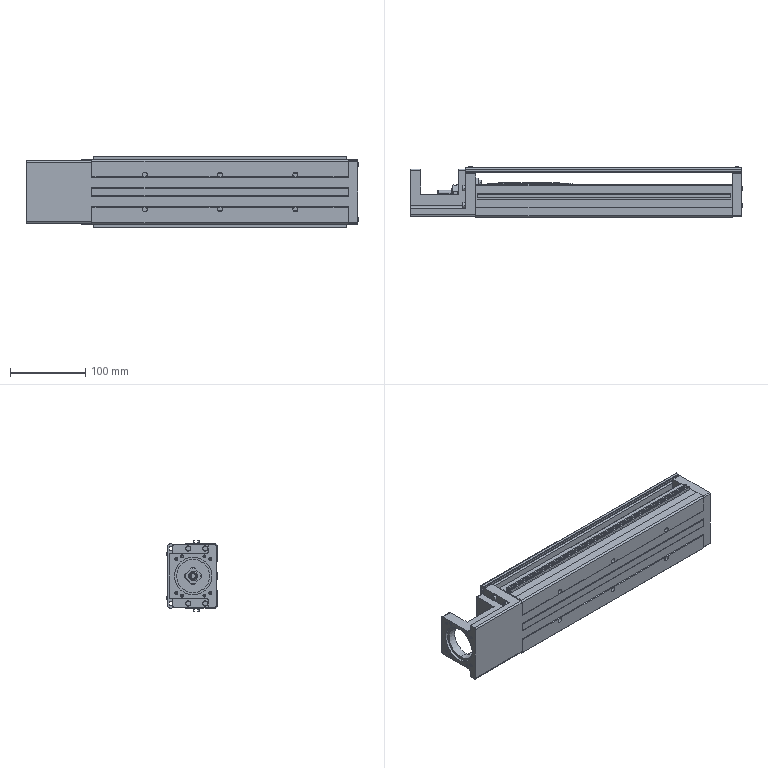Part | STEP file | 5 solids | 681 faces | box 440.5 x 67.1 x 95.1 mm | volume 1162435 mm3 | plane 307 | cylinder 220 | cone 130 | spline 24 | commonest cylinder face diameters 0.2 x24 5.5 x18 3.242 x16 2.113 x12 6.6 x12 7 x12